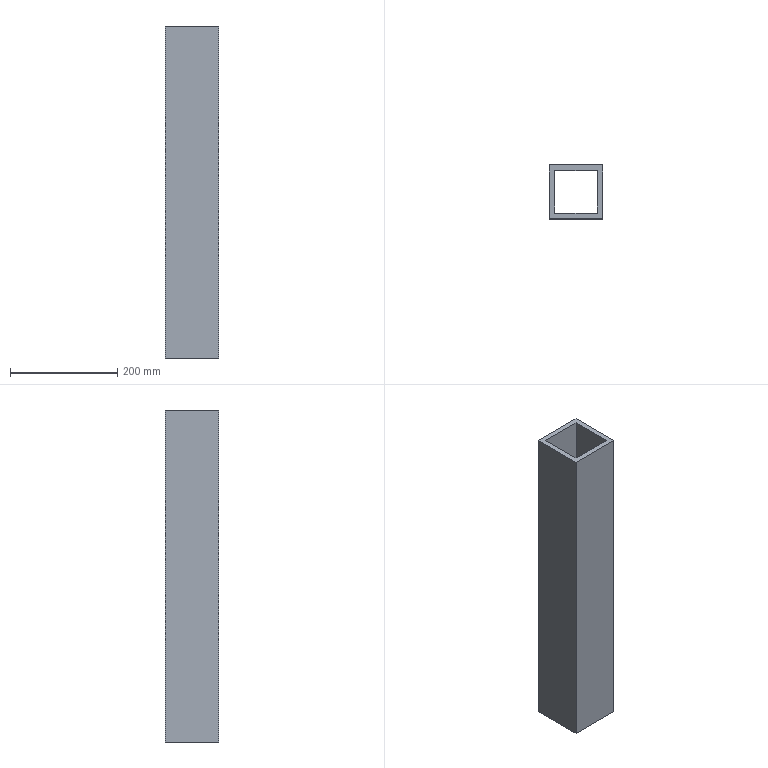Part | SolidWorks | features BaseBody 1 | 1 solid | 10 faces | box 100 x 100 x 620 mm | volume 2232000 mm3 | plane 10
STEP:
#1=CARTESIAN_POINT('',(-50.,50.,-310.));
#2=VERTEX_POINT('',#1);
#3=CARTESIAN_POINT('',(-50.,50.,310.));
#4=VERTEX_POINT('',#3);
#5=CARTESIAN_POINT('',(-50.,50.,-310.));
#6=DIRECTION('',(0.,0.,1.));
#7=VECTOR('',#6,1000.);
#8=LINE('',#5,#7);
#9=EDGE_CURVE('',#2,#4,#8,.T.);
#10=ORIENTED_EDGE('',*,*,#9,.F.);
#11=CARTESIAN_POINT('',(-50.,-50.,-310.));
#12=VERTEX_POINT('',#11);
#13=CARTESIAN_POINT('',(-50.,-50.,-310.));
#14=DIRECTION('',(0.,1.,0.));
#15=VECTOR('',#14,1000.);
#16=LINE('',#13,#15);
#17=EDGE_CURVE('',#12,#2,#16,.T.);
#18=ORIENTED_EDGE('',*,*,#17,.F.);
#19=CARTESIAN_POINT('',(-50.,-50.,310.));
#20=VERTEX_POINT('',#19);
#21=CARTESIAN_POINT('',(-50.,-50.,-310.));
#22=DIRECTION('',(0.,0.,-1.));
#23=VECTOR('',#22,1000.);
#24=LINE('',#21,#23);
#25=EDGE_CURVE('',#20,#12,#24,.T.);
#26=ORIENTED_EDGE('',*,*,#25,.F.);
#27=CARTESIAN_POINT('',(-50.,-50.,310.));
#28=DIRECTION('',(0.,-1.,0.));
#29=VECTOR('',#28,1000.);
#30=LINE('',#27,#29);
#31=EDGE_CURVE('',#4,#20,#30,.T.);
#32=ORIENTED_EDGE('',*,*,#31,.F.);
#33=EDGE_LOOP('',(#10,#18,#26,#32));
#34=FACE_OUTER_BOUND('',#33,.T.);
#35=CARTESIAN_POINT('',(-50.,-50.,-310.));
#36=DIRECTION('',(1.,0.,0.));
#37=DIRECTION('',(0.,0.,-1.));
#38=AXIS2_PLACEMENT_3D('',#35,#36,#37);
#39=PLANE('',#38);
#40=ADVANCED_FACE('',(#34),#39,.F.);
#41=CARTESIAN_POINT('',(-40.,40.,310.));
#42=VERTEX_POINT('',#41);
#43=CARTESIAN_POINT('',(40.,40.,310.));
#44=VERTEX_POINT('',#43);
#45=CARTESIAN_POINT('',(-50.,40.,310.));
#46=DIRECTION('',(1.,0.,0.));
#47=VECTOR('',#46,1000.);
#48=LINE('',#45,#47);
#49=EDGE_CURVE('',#42,#44,#48,.T.);
#50=ORIENTED_EDGE('',*,*,#49,.T.);
#51=CARTESIAN_POINT('',(40.,-40.,310.));
#52=VERTEX_POINT('',#51);
#53=CARTESIAN_POINT('',(40.,-50.,310.));
#54=DIRECTION('',(0.,-1.,0.));
#55=VECTOR('',#54,1000.);
#56=LINE('',#53,#55);
#57=EDGE_CURVE('',#44,#52,#56,.T.);
#58=ORIENTED_EDGE('',*,*,#57,.T.);
#59=CARTESIAN_POINT('',(-40.,-40.,310.));
#60=VERTEX_POINT('',#59);
#61=CARTESIAN_POINT('',(-50.,-40.,310.));
#62=DIRECTION('',(-1.,0.,0.));
#63=VECTOR('',#62,1000.);
#64=LINE('',#61,#63);
#65=EDGE_CURVE('',#52,#60,#64,.T.);
#66=ORIENTED_EDGE('',*,*,#65,.T.);
#67=CARTESIAN_POINT('',(-40.,-50.,310.));
#68=DIRECTION('',(0.,1.,0.));
#69=VECTOR('',#68,1000.);
#70=LINE('',#67,#69);
#71=EDGE_CURVE('',#60,#42,#70,.T.);
#72=ORIENTED_EDGE('',*,*,#71,.T.);
#73=EDGE_LOOP('',(#50,#58,#66,#72));
#74=FACE_BOUND('',#73,.T.);
#75=CARTESIAN_POINT('',(50.,-50.,310.));
#76=VERTEX_POINT('',#75);
#77=CARTESIAN_POINT('',(50.,50.,310.));
#78=VERTEX_POINT('',#77);
#79=CARTESIAN_POINT('',(50.,-50.,310.));
#80=DIRECTION('',(0.,1.,0.));
#81=VECTOR('',#80,1000.);
#82=LINE('',#79,#81);
#83=EDGE_CURVE('',#76,#78,#82,.T.);
#84=ORIENTED_EDGE('',*,*,#83,.T.);
#85=CARTESIAN_POINT('',(-50.,50.,310.));
#86=DIRECTION('',(-1.,0.,0.));
#87=VECTOR('',#86,1000.);
#88=LINE('',#85,#87);
#89=EDGE_CURVE('',#78,#4,#88,.T.);
#90=ORIENTED_EDGE('',*,*,#89,.T.);
#91=ORIENTED_EDGE('',*,*,#31,.T.);
#92=CARTESIAN_POINT('',(-50.,-50.,310.));
#93=DIRECTION('',(1.,0.,0.));
#94=VECTOR('',#93,1000.);
#95=LINE('',#92,#94);
#96=EDGE_CURVE('',#20,#76,#95,.T.);
#97=ORIENTED_EDGE('',*,*,#96,.T.);
#98=EDGE_LOOP('',(#84,#90,#91,#97));
#99=FACE_OUTER_BOUND('',#98,.T.);
#100=CARTESIAN_POINT('',(-50.,-50.,310.));
#101=DIRECTION('',(0.,0.,1.));
#102=DIRECTION('',(1.,0.,0.));
#103=AXIS2_PLACEMENT_3D('',#100,#101,#102);
#104=PLANE('',#103);
#105=ADVANCED_FACE('',(#74,#99),#104,.T.);
#106=ORIENTED_EDGE('',*,*,#89,.F.);
#107=CARTESIAN_POINT('',(50.,50.,-310.));
#108=VERTEX_POINT('',#107);
#109=CARTESIAN_POINT('',(50.,50.,-310.));
#110=DIRECTION('',(0.,0.,-1.));
#111=VECTOR('',#110,1000.);
#112=LINE('',#109,#111);
#113=EDGE_CURVE('',#78,#108,#112,.T.);
#114=ORIENTED_EDGE('',*,*,#113,.T.);
#115=CARTESIAN_POINT('',(-50.,50.,-310.));
#116=DIRECTION('',(-1.,0.,0.));
#117=VECTOR('',#116,1000.);
#118=LINE('',#115,#117);
#119=EDGE_CURVE('',#108,#2,#118,.T.);
#120=ORIENTED_EDGE('',*,*,#119,.T.);
#121=ORIENTED_EDGE('',*,*,#9,.T.);
#122=EDGE_LOOP('',(#106,#114,#120,#121));
#123=FACE_OUTER_BOUND('',#122,.T.);
#124=CARTESIAN_POINT('',(-50.,50.,-310.));
#125=DIRECTION('',(0.,1.,0.));
#126=DIRECTION('',(0.,0.,1.));
#127=AXIS2_PLACEMENT_3D('',#124,#125,#126);
#128=PLANE('',#127);
#129=ADVANCED_FACE('',(#123),#128,.T.);
#130=CARTESIAN_POINT('',(-40.,40.,-310.));
#131=VERTEX_POINT('',#130);
#132=CARTESIAN_POINT('',(40.,40.,-310.));
#133=VERTEX_POINT('',#132);
#134=CARTESIAN_POINT('',(-50.,40.,-310.));
#135=DIRECTION('',(1.,0.,0.));
#136=VECTOR('',#135,1000.);
#137=LINE('',#134,#136);
#138=EDGE_CURVE('',#131,#133,#137,.T.);
#139=ORIENTED_EDGE('',*,*,#138,.F.);
#140=CARTESIAN_POINT('',(-40.,-40.,-310.));
#141=VERTEX_POINT('',#140);
#142=CARTESIAN_POINT('',(-40.,-50.,-310.));
#143=DIRECTION('',(0.,1.,0.));
#144=VECTOR('',#143,1000.);
#145=LINE('',#142,#144);
#146=EDGE_CURVE('',#141,#131,#145,.T.);
#147=ORIENTED_EDGE('',*,*,#146,.F.);
#148=CARTESIAN_POINT('',(40.,-40.,-310.));
#149=VERTEX_POINT('',#148);
#150=CARTESIAN_POINT('',(-50.,-40.,-310.));
#151=DIRECTION('',(-1.,0.,0.));
#152=VECTOR('',#151,1000.);
#153=LINE('',#150,#152);
#154=EDGE_CURVE('',#149,#141,#153,.T.);
#155=ORIENTED_EDGE('',*,*,#154,.F.);
#156=CARTESIAN_POINT('',(40.,-50.,-310.));
#157=DIRECTION('',(0.,-1.,0.));
#158=VECTOR('',#157,1000.);
#159=LINE('',#156,#158);
#160=EDGE_CURVE('',#133,#149,#159,.T.);
#161=ORIENTED_EDGE('',*,*,#160,.F.);
#162=EDGE_LOOP('',(#139,#147,#155,#161));
#163=FACE_BOUND('',#162,.T.);
#164=CARTESIAN_POINT('',(50.,-50.,-310.));
#165=VERTEX_POINT('',#164);
#166=CARTESIAN_POINT('',(50.,-50.,-310.));
#167=DIRECTION('',(0.,1.,0.));
#168=VECTOR('',#167,1000.);
#169=LINE('',#166,#168);
#170=EDGE_CURVE('',#165,#108,#169,.T.);
#171=ORIENTED_EDGE('',*,*,#170,.F.);
#172=CARTESIAN_POINT('',(-50.,-50.,-310.));
#173=DIRECTION('',(1.,0.,0.));
#174=VECTOR('',#173,1000.);
#175=LINE('',#172,#174);
#176=EDGE_CURVE('',#12,#165,#175,.T.);
#177=ORIENTED_EDGE('',*,*,#176,.F.);
#178=ORIENTED_EDGE('',*,*,#17,.T.);
#179=ORIENTED_EDGE('',*,*,#119,.F.);
#180=EDGE_LOOP('',(#171,#177,#178,#179));
#181=FACE_OUTER_BOUND('',#180,.T.);
#182=CARTESIAN_POINT('',(-50.,-50.,-310.));
#183=DIRECTION('',(0.,0.,1.));
#184=DIRECTION('',(1.,0.,0.));
#185=AXIS2_PLACEMENT_3D('',#182,#183,#184);
#186=PLANE('',#185);
#187=ADVANCED_FACE('',(#163,#181),#186,.F.);
#188=ORIENTED_EDGE('',*,*,#96,.F.);
#189=ORIENTED_EDGE('',*,*,#25,.T.);
#190=ORIENTED_EDGE('',*,*,#176,.T.);
#191=CARTESIAN_POINT('',(50.,-50.,-310.));
#192=DIRECTION('',(0.,0.,-1.));
#193=VECTOR('',#192,1000.);
#194=LINE('',#191,#193);
#195=EDGE_CURVE('',#76,#165,#194,.T.);
#196=ORIENTED_EDGE('',*,*,#195,.F.);
#197=EDGE_LOOP('',(#188,#189,#190,#196));
#198=FACE_OUTER_BOUND('',#197,.T.);
#199=CARTESIAN_POINT('',(-50.,-50.,-310.));
#200=DIRECTION('',(0.,1.,0.));
#201=DIRECTION('',(0.,0.,1.));
#202=AXIS2_PLACEMENT_3D('',#199,#200,#201);
#203=PLANE('',#202);
#204=ADVANCED_FACE('',(#198),#203,.F.);
#205=CARTESIAN_POINT('',(40.,40.,-311.));
#206=DIRECTION('',(0.,0.,1.));
#207=VECTOR('',#206,1000.);
#208=LINE('',#205,#207);
#209=EDGE_CURVE('',#133,#44,#208,.T.);
#210=ORIENTED_EDGE('',*,*,#209,.F.);
#211=ORIENTED_EDGE('',*,*,#160,.T.);
#212=CARTESIAN_POINT('',(40.,-40.,-311.));
#213=DIRECTION('',(0.,0.,-1.));
#214=VECTOR('',#213,1000.);
#215=LINE('',#212,#214);
#216=EDGE_CURVE('',#52,#149,#215,.T.);
#217=ORIENTED_EDGE('',*,*,#216,.F.);
#218=ORIENTED_EDGE('',*,*,#57,.F.);
#219=EDGE_LOOP('',(#210,#211,#217,#218));
#220=FACE_OUTER_BOUND('',#219,.T.);
#221=CARTESIAN_POINT('',(40.,-40.,-311.));
#222=DIRECTION('',(1.,0.,0.));
#223=DIRECTION('',(0.,0.,-1.));
#224=AXIS2_PLACEMENT_3D('',#221,#222,#223);
#225=PLANE('',#224);
#226=ADVANCED_FACE('',(#220),#225,.F.);
#227=CARTESIAN_POINT('',(-40.,40.,-311.));
#228=DIRECTION('',(0.,0.,1.));
#229=VECTOR('',#228,1000.);
#230=LINE('',#227,#229);
#231=EDGE_CURVE('',#131,#42,#230,.T.);
#232=ORIENTED_EDGE('',*,*,#231,.F.);
#233=ORIENTED_EDGE('',*,*,#138,.T.);
#234=ORIENTED_EDGE('',*,*,#209,.T.);
#235=ORIENTED_EDGE('',*,*,#49,.F.);
#236=EDGE_LOOP('',(#232,#233,#234,#235));
#237=FACE_OUTER_BOUND('',#236,.T.);
#238=CARTESIAN_POINT('',(-40.,40.,-311.));
#239=DIRECTION('',(0.,1.,0.));
#240=DIRECTION('',(0.,0.,1.));
#241=AXIS2_PLACEMENT_3D('',#238,#239,#240);
#242=PLANE('',#241);
#243=ADVANCED_FACE('',(#237),#242,.F.);
#244=ORIENTED_EDGE('',*,*,#231,.T.);
#245=ORIENTED_EDGE('',*,*,#71,.F.);
#246=CARTESIAN_POINT('',(-40.,-40.,-311.));
#247=DIRECTION('',(0.,0.,-1.));
#248=VECTOR('',#247,1000.);
#249=LINE('',#246,#248);
#250=EDGE_CURVE('',#60,#141,#249,.T.);
#251=ORIENTED_EDGE('',*,*,#250,.T.);
#252=ORIENTED_EDGE('',*,*,#146,.T.);
#253=EDGE_LOOP('',(#244,#245,#251,#252));
#254=FACE_OUTER_BOUND('',#253,.T.);
#255=CARTESIAN_POINT('',(-40.,-40.,-311.));
#256=DIRECTION('',(1.,0.,0.));
#257=DIRECTION('',(0.,0.,-1.));
#258=AXIS2_PLACEMENT_3D('',#255,#256,#257);
#259=PLANE('',#258);
#260=ADVANCED_FACE('',(#254),#259,.T.);
#261=ORIENTED_EDGE('',*,*,#250,.F.);
#262=ORIENTED_EDGE('',*,*,#65,.F.);
#263=ORIENTED_EDGE('',*,*,#216,.T.);
#264=ORIENTED_EDGE('',*,*,#154,.T.);
#265=EDGE_LOOP('',(#261,#262,#263,#264));
#266=FACE_OUTER_BOUND('',#265,.T.);
#267=CARTESIAN_POINT('',(-40.,-40.,-311.));
#268=DIRECTION('',(0.,1.,0.));
#269=DIRECTION('',(0.,0.,1.));
#270=AXIS2_PLACEMENT_3D('',#267,#268,#269);
#271=PLANE('',#270);
#272=ADVANCED_FACE('',(#266),#271,.T.);
#273=ORIENTED_EDGE('',*,*,#113,.F.);
#274=ORIENTED_EDGE('',*,*,#83,.F.);
#275=ORIENTED_EDGE('',*,*,#195,.T.);
#276=ORIENTED_EDGE('',*,*,#170,.T.);
#277=EDGE_LOOP('',(#273,#274,#275,#276));
#278=FACE_OUTER_BOUND('',#277,.T.);
#279=CARTESIAN_POINT('',(50.,-50.,-310.));
#280=DIRECTION('',(1.,0.,0.));
#281=DIRECTION('',(0.,0.,-1.));
#282=AXIS2_PLACEMENT_3D('',#279,#280,#281);
#283=PLANE('',#282);
#284=ADVANCED_FACE('',(#278),#283,.T.);
#285=CLOSED_SHELL('',(#40,#105,#129,#187,#204,#226,#243,#260,#272,#284));
#286=MANIFOLD_SOLID_BREP('',#285);
#287=CARTESIAN_POINT('',(0.,0.,0.));
#288=DIRECTION('',(0.,0.,1.));
#289=DIRECTION('',(1.,0.,0.));
#290=AXIS2_PLACEMENT_3D('',#287,#288,#289);
#291=(LENGTH_UNIT()NAMED_UNIT(*)SI_UNIT(.MILLI.,.METRE.));
#292=UNCERTAINTY_MEASURE_WITH_UNIT(LENGTH_MEASURE(0.00001),#291,'','');
#293=(NAMED_UNIT(*)PLANE_ANGLE_UNIT()SI_UNIT($,.RADIAN.));
#294=(NAMED_UNIT(*)SI_UNIT($,.STERADIAN.)SOLID_ANGLE_UNIT());
#295=(GEOMETRIC_REPRESENTATION_CONTEXT(3)GLOBAL_UNCERTAINTY_ASSIGNED_CONTEXT((#292))GLOBAL_UNIT_ASSIGNED_CONTEXT((#291,#293,#294))REPRESENTATION_CONTEXT('',''));
#296=ADVANCED_BREP_SHAPE_REPRESENTATION('',(#286,#290),#295);